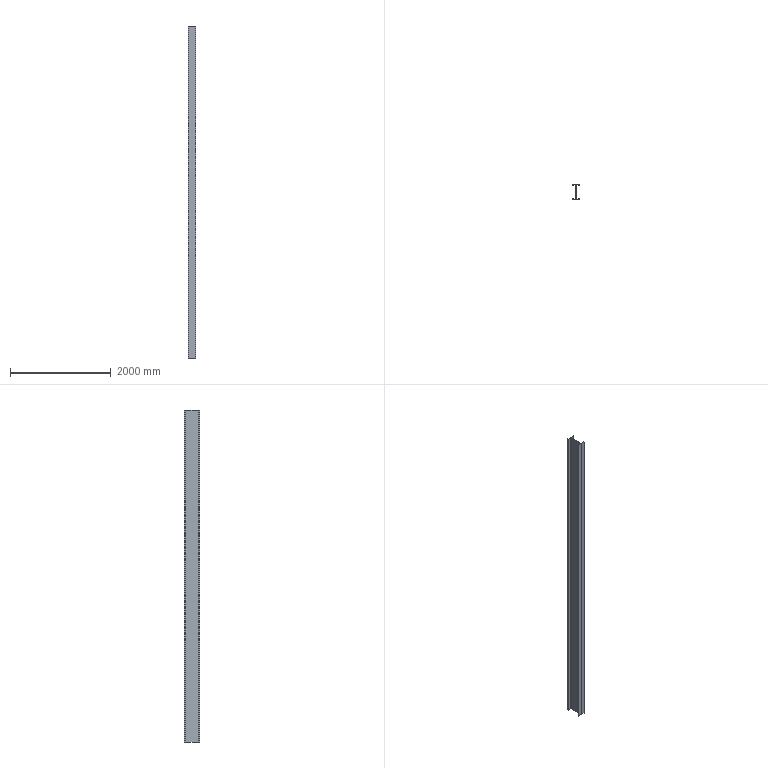Part | SolidWorks | features Extrusion 1 | 1 solid | 18 faces | box 150 x 300 x 6592 mm | volume 30837843 mm3 | plane 14 | cylinder 4 | commonest cylinder face diameters 26 x4
STEP:
#1=CARTESIAN_POINT('',(-75.,9.,0.));
#2=VERTEX_POINT('',#1);
#3=CARTESIAN_POINT('',(-75.,0.,0.));
#4=VERTEX_POINT('',#3);
#5=CARTESIAN_POINT('',(-75.,0.,0.));
#6=DIRECTION('',(0.,-1.,0.));
#7=VECTOR('',#6,1000.);
#8=LINE('',#5,#7);
#9=EDGE_CURVE('',#2,#4,#8,.T.);
#10=ORIENTED_EDGE('',*,*,#9,.T.);
#11=CARTESIAN_POINT('',(-75.,0.,6592.));
#12=VERTEX_POINT('',#11);
#13=CARTESIAN_POINT('',(-75.,0.,6592.));
#14=DIRECTION('',(0.,0.,-1.));
#15=VECTOR('',#14,1000.);
#16=LINE('',#13,#15);
#17=EDGE_CURVE('',#12,#4,#16,.T.);
#18=ORIENTED_EDGE('',*,*,#17,.F.);
#19=CARTESIAN_POINT('',(-75.,9.,6592.));
#20=VERTEX_POINT('',#19);
#21=CARTESIAN_POINT('',(-75.,0.,6592.));
#22=DIRECTION('',(0.,-1.,0.));
#23=VECTOR('',#22,1000.);
#24=LINE('',#21,#23);
#25=EDGE_CURVE('',#20,#12,#24,.T.);
#26=ORIENTED_EDGE('',*,*,#25,.F.);
#27=CARTESIAN_POINT('',(-75.,9.,6592.));
#28=DIRECTION('',(0.,0.,-1.));
#29=VECTOR('',#28,1000.);
#30=LINE('',#27,#29);
#31=EDGE_CURVE('',#20,#2,#30,.T.);
#32=ORIENTED_EDGE('',*,*,#31,.T.);
#33=EDGE_LOOP('',(#10,#18,#26,#32));
#34=FACE_OUTER_BOUND('',#33,.T.);
#35=CARTESIAN_POINT('',(-75.,0.,6592.));
#36=DIRECTION('',(1.,0.,0.));
#37=DIRECTION('',(0.,0.,-1.));
#38=AXIS2_PLACEMENT_3D('',#35,#36,#37);
#39=PLANE('',#38);
#40=ADVANCED_FACE('',(#34),#39,.F.);
#41=CARTESIAN_POINT('',(75.,0.,0.));
#42=VERTEX_POINT('',#41);
#43=CARTESIAN_POINT('',(75.,0.,0.));
#44=DIRECTION('',(1.,0.,0.));
#45=VECTOR('',#44,1000.);
#46=LINE('',#43,#45);
#47=EDGE_CURVE('',#4,#42,#46,.T.);
#48=ORIENTED_EDGE('',*,*,#47,.T.);
#49=CARTESIAN_POINT('',(75.,0.,6592.));
#50=VERTEX_POINT('',#49);
#51=CARTESIAN_POINT('',(75.,0.,6592.));
#52=DIRECTION('',(0.,0.,-1.));
#53=VECTOR('',#52,1000.);
#54=LINE('',#51,#53);
#55=EDGE_CURVE('',#50,#42,#54,.T.);
#56=ORIENTED_EDGE('',*,*,#55,.F.);
#57=CARTESIAN_POINT('',(75.,0.,6592.));
#58=DIRECTION('',(1.,0.,0.));
#59=VECTOR('',#58,1000.);
#60=LINE('',#57,#59);
#61=EDGE_CURVE('',#12,#50,#60,.T.);
#62=ORIENTED_EDGE('',*,*,#61,.F.);
#63=ORIENTED_EDGE('',*,*,#17,.T.);
#64=EDGE_LOOP('',(#48,#56,#62,#63));
#65=FACE_OUTER_BOUND('',#64,.T.);
#66=CARTESIAN_POINT('',(75.,0.,6592.));
#67=DIRECTION('',(0.,1.,0.));
#68=DIRECTION('',(-1.,0.,0.));
#69=AXIS2_PLACEMENT_3D('',#66,#67,#68);
#70=PLANE('',#69);
#71=ADVANCED_FACE('',(#65),#70,.F.);
#72=CARTESIAN_POINT('',(75.,9.,0.));
#73=VERTEX_POINT('',#72);
#74=CARTESIAN_POINT('',(75.,0.,0.));
#75=DIRECTION('',(0.,1.,0.));
#76=VECTOR('',#75,1000.);
#77=LINE('',#74,#76);
#78=EDGE_CURVE('',#42,#73,#77,.T.);
#79=ORIENTED_EDGE('',*,*,#78,.T.);
#80=CARTESIAN_POINT('',(75.,9.,6592.));
#81=VERTEX_POINT('',#80);
#82=CARTESIAN_POINT('',(75.,9.,6592.));
#83=DIRECTION('',(0.,0.,-1.));
#84=VECTOR('',#83,1000.);
#85=LINE('',#82,#84);
#86=EDGE_CURVE('',#81,#73,#85,.T.);
#87=ORIENTED_EDGE('',*,*,#86,.F.);
#88=CARTESIAN_POINT('',(75.,0.,6592.));
#89=DIRECTION('',(0.,1.,0.));
#90=VECTOR('',#89,1000.);
#91=LINE('',#88,#90);
#92=EDGE_CURVE('',#50,#81,#91,.T.);
#93=ORIENTED_EDGE('',*,*,#92,.F.);
#94=ORIENTED_EDGE('',*,*,#55,.T.);
#95=EDGE_LOOP('',(#79,#87,#93,#94));
#96=FACE_OUTER_BOUND('',#95,.T.);
#97=CARTESIAN_POINT('',(75.,0.,6592.));
#98=DIRECTION('',(-1.,0.,0.));
#99=DIRECTION('',(0.,0.,1.));
#100=AXIS2_PLACEMENT_3D('',#97,#98,#99);
#101=PLANE('',#100);
#102=ADVANCED_FACE('',(#96),#101,.F.);
#103=CARTESIAN_POINT('',(16.25,9.,0.));
#104=VERTEX_POINT('',#103);
#105=CARTESIAN_POINT('',(75.,9.,0.));
#106=DIRECTION('',(-1.,0.,0.));
#107=VECTOR('',#106,1000.);
#108=LINE('',#105,#107);
#109=EDGE_CURVE('',#73,#104,#108,.T.);
#110=ORIENTED_EDGE('',*,*,#109,.T.);
#111=CARTESIAN_POINT('',(16.25,9.,6592.));
#112=VERTEX_POINT('',#111);
#113=CARTESIAN_POINT('',(16.25,9.,6592.));
#114=DIRECTION('',(0.,0.,-1.));
#115=VECTOR('',#114,1000.);
#116=LINE('',#113,#115);
#117=EDGE_CURVE('',#112,#104,#116,.T.);
#118=ORIENTED_EDGE('',*,*,#117,.F.);
#119=CARTESIAN_POINT('',(75.,9.,6592.));
#120=DIRECTION('',(-1.,0.,0.));
#121=VECTOR('',#120,1000.);
#122=LINE('',#119,#121);
#123=EDGE_CURVE('',#81,#112,#122,.T.);
#124=ORIENTED_EDGE('',*,*,#123,.F.);
#125=ORIENTED_EDGE('',*,*,#86,.T.);
#126=EDGE_LOOP('',(#110,#118,#124,#125));
#127=FACE_OUTER_BOUND('',#126,.T.);
#128=CARTESIAN_POINT('',(75.,9.,6592.));
#129=DIRECTION('',(0.,-1.,0.));
#130=DIRECTION('',(1.,0.,0.));
#131=AXIS2_PLACEMENT_3D('',#128,#129,#130);
#132=PLANE('',#131);
#133=ADVANCED_FACE('',(#127),#132,.F.);
#134=CARTESIAN_POINT('',(3.25,22.,0.));
#135=VERTEX_POINT('',#134);
#136=CARTESIAN_POINT('',(16.25,22.,0.));
#137=DIRECTION('',(0.,0.,-1.));
#138=DIRECTION('',(-1.,0.,0.));
#139=AXIS2_PLACEMENT_3D('',#136,#137,#138);
#140=CIRCLE('',#139,13.);
#141=EDGE_CURVE('',#104,#135,#140,.T.);
#142=ORIENTED_EDGE('',*,*,#141,.T.);
#143=CARTESIAN_POINT('',(3.25,22.,6592.));
#144=VERTEX_POINT('',#143);
#145=CARTESIAN_POINT('',(3.25,22.,6592.));
#146=DIRECTION('',(0.,0.,-1.));
#147=VECTOR('',#146,1000.);
#148=LINE('',#145,#147);
#149=EDGE_CURVE('',#144,#135,#148,.T.);
#150=ORIENTED_EDGE('',*,*,#149,.F.);
#151=CARTESIAN_POINT('',(16.25,22.,6592.));
#152=DIRECTION('',(0.,0.,-1.));
#153=DIRECTION('',(-1.,0.,0.));
#154=AXIS2_PLACEMENT_3D('',#151,#152,#153);
#155=CIRCLE('',#154,13.);
#156=EDGE_CURVE('',#112,#144,#155,.T.);
#157=ORIENTED_EDGE('',*,*,#156,.F.);
#158=ORIENTED_EDGE('',*,*,#117,.T.);
#159=EDGE_LOOP('',(#142,#150,#157,#158));
#160=FACE_OUTER_BOUND('',#159,.T.);
#161=CARTESIAN_POINT('',(16.25,22.,6592.));
#162=DIRECTION('',(0.,0.,-1.));
#163=DIRECTION('',(-1.,0.,0.));
#164=AXIS2_PLACEMENT_3D('',#161,#162,#163);
#165=CYLINDRICAL_SURFACE('',#164,13.);
#166=ADVANCED_FACE('',(#160),#165,.F.);
#167=CARTESIAN_POINT('',(3.25,278.,0.));
#168=VERTEX_POINT('',#167);
#169=CARTESIAN_POINT('',(3.25,22.,0.));
#170=DIRECTION('',(0.,1.,0.));
#171=VECTOR('',#170,1000.);
#172=LINE('',#169,#171);
#173=EDGE_CURVE('',#135,#168,#172,.T.);
#174=ORIENTED_EDGE('',*,*,#173,.T.);
#175=CARTESIAN_POINT('',(3.25,278.,6592.));
#176=VERTEX_POINT('',#175);
#177=CARTESIAN_POINT('',(3.25,278.,6592.));
#178=DIRECTION('',(0.,0.,-1.));
#179=VECTOR('',#178,1000.);
#180=LINE('',#177,#179);
#181=EDGE_CURVE('',#176,#168,#180,.T.);
#182=ORIENTED_EDGE('',*,*,#181,.F.);
#183=CARTESIAN_POINT('',(3.25,22.,6592.));
#184=DIRECTION('',(0.,1.,0.));
#185=VECTOR('',#184,1000.);
#186=LINE('',#183,#185);
#187=EDGE_CURVE('',#144,#176,#186,.T.);
#188=ORIENTED_EDGE('',*,*,#187,.F.);
#189=ORIENTED_EDGE('',*,*,#149,.T.);
#190=EDGE_LOOP('',(#174,#182,#188,#189));
#191=FACE_OUTER_BOUND('',#190,.T.);
#192=CARTESIAN_POINT('',(3.25,22.,6592.));
#193=DIRECTION('',(-1.,0.,0.));
#194=DIRECTION('',(0.,0.,1.));
#195=AXIS2_PLACEMENT_3D('',#192,#193,#194);
#196=PLANE('',#195);
#197=ADVANCED_FACE('',(#191),#196,.F.);
#198=CARTESIAN_POINT('',(16.25,291.,0.));
#199=VERTEX_POINT('',#198);
#200=CARTESIAN_POINT('',(16.25,278.,0.));
#201=DIRECTION('',(0.,0.,-1.));
#202=DIRECTION('',(-1.,0.,0.));
#203=AXIS2_PLACEMENT_3D('',#200,#201,#202);
#204=CIRCLE('',#203,13.);
#205=EDGE_CURVE('',#168,#199,#204,.T.);
#206=ORIENTED_EDGE('',*,*,#205,.T.);
#207=CARTESIAN_POINT('',(16.25,291.,6592.));
#208=VERTEX_POINT('',#207);
#209=CARTESIAN_POINT('',(16.25,291.,6592.));
#210=DIRECTION('',(0.,0.,-1.));
#211=VECTOR('',#210,1000.);
#212=LINE('',#209,#211);
#213=EDGE_CURVE('',#208,#199,#212,.T.);
#214=ORIENTED_EDGE('',*,*,#213,.F.);
#215=CARTESIAN_POINT('',(16.25,278.,6592.));
#216=DIRECTION('',(0.,0.,-1.));
#217=DIRECTION('',(-1.,0.,0.));
#218=AXIS2_PLACEMENT_3D('',#215,#216,#217);
#219=CIRCLE('',#218,13.);
#220=EDGE_CURVE('',#176,#208,#219,.T.);
#221=ORIENTED_EDGE('',*,*,#220,.F.);
#222=ORIENTED_EDGE('',*,*,#181,.T.);
#223=EDGE_LOOP('',(#206,#214,#221,#222));
#224=FACE_OUTER_BOUND('',#223,.T.);
#225=CARTESIAN_POINT('',(16.25,278.,6592.));
#226=DIRECTION('',(0.,0.,-1.));
#227=DIRECTION('',(-1.,0.,0.));
#228=AXIS2_PLACEMENT_3D('',#225,#226,#227);
#229=CYLINDRICAL_SURFACE('',#228,13.);
#230=ADVANCED_FACE('',(#224),#229,.F.);
#231=CARTESIAN_POINT('',(75.,291.,0.));
#232=VERTEX_POINT('',#231);
#233=CARTESIAN_POINT('',(16.25,291.,0.));
#234=DIRECTION('',(1.,0.,0.));
#235=VECTOR('',#234,1000.);
#236=LINE('',#233,#235);
#237=EDGE_CURVE('',#199,#232,#236,.T.);
#238=ORIENTED_EDGE('',*,*,#237,.T.);
#239=CARTESIAN_POINT('',(75.,291.,6592.));
#240=VERTEX_POINT('',#239);
#241=CARTESIAN_POINT('',(75.,291.,6592.));
#242=DIRECTION('',(0.,0.,-1.));
#243=VECTOR('',#242,1000.);
#244=LINE('',#241,#243);
#245=EDGE_CURVE('',#240,#232,#244,.T.);
#246=ORIENTED_EDGE('',*,*,#245,.F.);
#247=CARTESIAN_POINT('',(16.25,291.,6592.));
#248=DIRECTION('',(1.,0.,0.));
#249=VECTOR('',#248,1000.);
#250=LINE('',#247,#249);
#251=EDGE_CURVE('',#208,#240,#250,.T.);
#252=ORIENTED_EDGE('',*,*,#251,.F.);
#253=ORIENTED_EDGE('',*,*,#213,.T.);
#254=EDGE_LOOP('',(#238,#246,#252,#253));
#255=FACE_OUTER_BOUND('',#254,.T.);
#256=CARTESIAN_POINT('',(16.25,291.,6592.));
#257=DIRECTION('',(0.,1.,0.));
#258=DIRECTION('',(-1.,0.,0.));
#259=AXIS2_PLACEMENT_3D('',#256,#257,#258);
#260=PLANE('',#259);
#261=ADVANCED_FACE('',(#255),#260,.F.);
#262=CARTESIAN_POINT('',(75.,300.,0.));
#263=VERTEX_POINT('',#262);
#264=CARTESIAN_POINT('',(75.,291.,0.));
#265=DIRECTION('',(0.,1.,0.));
#266=VECTOR('',#265,1000.);
#267=LINE('',#264,#266);
#268=EDGE_CURVE('',#232,#263,#267,.T.);
#269=ORIENTED_EDGE('',*,*,#268,.T.);
#270=CARTESIAN_POINT('',(75.,300.,6592.));
#271=VERTEX_POINT('',#270);
#272=CARTESIAN_POINT('',(75.,300.,6592.));
#273=DIRECTION('',(0.,0.,-1.));
#274=VECTOR('',#273,1000.);
#275=LINE('',#272,#274);
#276=EDGE_CURVE('',#271,#263,#275,.T.);
#277=ORIENTED_EDGE('',*,*,#276,.F.);
#278=CARTESIAN_POINT('',(75.,291.,6592.));
#279=DIRECTION('',(0.,1.,0.));
#280=VECTOR('',#279,1000.);
#281=LINE('',#278,#280);
#282=EDGE_CURVE('',#240,#271,#281,.T.);
#283=ORIENTED_EDGE('',*,*,#282,.F.);
#284=ORIENTED_EDGE('',*,*,#245,.T.);
#285=EDGE_LOOP('',(#269,#277,#283,#284));
#286=FACE_OUTER_BOUND('',#285,.T.);
#287=CARTESIAN_POINT('',(75.,291.,6592.));
#288=DIRECTION('',(-1.,0.,0.));
#289=DIRECTION('',(0.,-1.,0.));
#290=AXIS2_PLACEMENT_3D('',#287,#288,#289);
#291=PLANE('',#290);
#292=ADVANCED_FACE('',(#286),#291,.F.);
#293=CARTESIAN_POINT('',(-75.,300.,0.));
#294=VERTEX_POINT('',#293);
#295=CARTESIAN_POINT('',(-75.,300.,0.));
#296=DIRECTION('',(-1.,0.,0.));
#297=VECTOR('',#296,1000.);
#298=LINE('',#295,#297);
#299=EDGE_CURVE('',#263,#294,#298,.T.);
#300=ORIENTED_EDGE('',*,*,#299,.T.);
#301=CARTESIAN_POINT('',(-75.,300.,6592.));
#302=VERTEX_POINT('',#301);
#303=CARTESIAN_POINT('',(-75.,300.,6592.));
#304=DIRECTION('',(0.,0.,-1.));
#305=VECTOR('',#304,1000.);
#306=LINE('',#303,#305);
#307=EDGE_CURVE('',#302,#294,#306,.T.);
#308=ORIENTED_EDGE('',*,*,#307,.F.);
#309=CARTESIAN_POINT('',(-75.,300.,6592.));
#310=DIRECTION('',(-1.,0.,0.));
#311=VECTOR('',#310,1000.);
#312=LINE('',#309,#311);
#313=EDGE_CURVE('',#271,#302,#312,.T.);
#314=ORIENTED_EDGE('',*,*,#313,.F.);
#315=ORIENTED_EDGE('',*,*,#276,.T.);
#316=EDGE_LOOP('',(#300,#308,#314,#315));
#317=FACE_OUTER_BOUND('',#316,.T.);
#318=CARTESIAN_POINT('',(-75.,300.,6592.));
#319=DIRECTION('',(0.,-1.,0.));
#320=DIRECTION('',(0.,0.,-1.));
#321=AXIS2_PLACEMENT_3D('',#318,#319,#320);
#322=PLANE('',#321);
#323=ADVANCED_FACE('',(#317),#322,.F.);
#324=CARTESIAN_POINT('',(-75.,291.,0.));
#325=VERTEX_POINT('',#324);
#326=CARTESIAN_POINT('',(-75.,291.,0.));
#327=DIRECTION('',(0.,-1.,0.));
#328=VECTOR('',#327,1000.);
#329=LINE('',#326,#328);
#330=EDGE_CURVE('',#294,#325,#329,.T.);
#331=ORIENTED_EDGE('',*,*,#330,.T.);
#332=CARTESIAN_POINT('',(-75.,291.,6592.));
#333=VERTEX_POINT('',#332);
#334=CARTESIAN_POINT('',(-75.,291.,6592.));
#335=DIRECTION('',(0.,0.,-1.));
#336=VECTOR('',#335,1000.);
#337=LINE('',#334,#336);
#338=EDGE_CURVE('',#333,#325,#337,.T.);
#339=ORIENTED_EDGE('',*,*,#338,.F.);
#340=CARTESIAN_POINT('',(-75.,291.,6592.));
#341=DIRECTION('',(0.,-1.,0.));
#342=VECTOR('',#341,1000.);
#343=LINE('',#340,#342);
#344=EDGE_CURVE('',#302,#333,#343,.T.);
#345=ORIENTED_EDGE('',*,*,#344,.F.);
#346=ORIENTED_EDGE('',*,*,#307,.T.);
#347=EDGE_LOOP('',(#331,#339,#345,#346));
#348=FACE_OUTER_BOUND('',#347,.T.);
#349=CARTESIAN_POINT('',(-75.,291.,6592.));
#350=DIRECTION('',(1.,0.,0.));
#351=DIRECTION('',(0.,1.,0.));
#352=AXIS2_PLACEMENT_3D('',#349,#350,#351);
#353=PLANE('',#352);
#354=ADVANCED_FACE('',(#348),#353,.F.);
#355=CARTESIAN_POINT('',(-16.25,291.,0.));
#356=VERTEX_POINT('',#355);
#357=CARTESIAN_POINT('',(-16.25,291.,0.));
#358=DIRECTION('',(1.,0.,0.));
#359=VECTOR('',#358,1000.);
#360=LINE('',#357,#359);
#361=EDGE_CURVE('',#325,#356,#360,.T.);
#362=ORIENTED_EDGE('',*,*,#361,.T.);
#363=CARTESIAN_POINT('',(-16.25,291.,6592.));
#364=VERTEX_POINT('',#363);
#365=CARTESIAN_POINT('',(-16.25,291.,6592.));
#366=DIRECTION('',(0.,0.,-1.));
#367=VECTOR('',#366,1000.);
#368=LINE('',#365,#367);
#369=EDGE_CURVE('',#364,#356,#368,.T.);
#370=ORIENTED_EDGE('',*,*,#369,.F.);
#371=CARTESIAN_POINT('',(-16.25,291.,6592.));
#372=DIRECTION('',(1.,0.,0.));
#373=VECTOR('',#372,1000.);
#374=LINE('',#371,#373);
#375=EDGE_CURVE('',#333,#364,#374,.T.);
#376=ORIENTED_EDGE('',*,*,#375,.F.);
#377=ORIENTED_EDGE('',*,*,#338,.T.);
#378=EDGE_LOOP('',(#362,#370,#376,#377));
#379=FACE_OUTER_BOUND('',#378,.T.);
#380=CARTESIAN_POINT('',(-16.25,291.,6592.));
#381=DIRECTION('',(0.,1.,0.));
#382=DIRECTION('',(-1.,0.,0.));
#383=AXIS2_PLACEMENT_3D('',#380,#381,#382);
#384=PLANE('',#383);
#385=ADVANCED_FACE('',(#379),#384,.F.);
#386=CARTESIAN_POINT('',(-3.25,278.,0.));
#387=VERTEX_POINT('',#386);
#388=CARTESIAN_POINT('',(-16.25,278.,0.));
#389=DIRECTION('',(0.,0.,-1.));
#390=DIRECTION('',(1.,0.,0.));
#391=AXIS2_PLACEMENT_3D('',#388,#389,#390);
#392=CIRCLE('',#391,13.);
#393=EDGE_CURVE('',#356,#387,#392,.T.);
#394=ORIENTED_EDGE('',*,*,#393,.T.);
#395=CARTESIAN_POINT('',(-3.25,278.,6592.));
#396=VERTEX_POINT('',#395);
#397=CARTESIAN_POINT('',(-3.25,278.,6592.));
#398=DIRECTION('',(0.,0.,-1.));
#399=VECTOR('',#398,1000.);
#400=LINE('',#397,#399);
#401=EDGE_CURVE('',#396,#387,#400,.T.);
#402=ORIENTED_EDGE('',*,*,#401,.F.);
#403=CARTESIAN_POINT('',(-16.25,278.,6592.));
#404=DIRECTION('',(0.,0.,-1.));
#405=DIRECTION('',(1.,0.,0.));
#406=AXIS2_PLACEMENT_3D('',#403,#404,#405);
#407=CIRCLE('',#406,13.);
#408=EDGE_CURVE('',#364,#396,#407,.T.);
#409=ORIENTED_EDGE('',*,*,#408,.F.);
#410=ORIENTED_EDGE('',*,*,#369,.T.);
#411=EDGE_LOOP('',(#394,#402,#409,#410));
#412=FACE_OUTER_BOUND('',#411,.T.);
#413=CARTESIAN_POINT('',(-16.25,278.,6592.));
#414=DIRECTION('',(0.,0.,-1.));
#415=DIRECTION('',(-1.,0.,0.));
#416=AXIS2_PLACEMENT_3D('',#413,#414,#415);
#417=CYLINDRICAL_SURFACE('',#416,13.);
#418=ADVANCED_FACE('',(#412),#417,.F.);
#419=CARTESIAN_POINT('',(-3.25,22.,0.));
#420=VERTEX_POINT('',#419);
#421=CARTESIAN_POINT('',(-3.25,22.,0.));
#422=DIRECTION('',(0.,-1.,0.));
#423=VECTOR('',#422,1000.);
#424=LINE('',#421,#423);
#425=EDGE_CURVE('',#387,#420,#424,.T.);
#426=ORIENTED_EDGE('',*,*,#425,.T.);
#427=CARTESIAN_POINT('',(-3.25,22.,6592.));
#428=VERTEX_POINT('',#427);
#429=CARTESIAN_POINT('',(-3.25,22.,6592.));
#430=DIRECTION('',(0.,0.,-1.));
#431=VECTOR('',#430,1000.);
#432=LINE('',#429,#431);
#433=EDGE_CURVE('',#428,#420,#432,.T.);
#434=ORIENTED_EDGE('',*,*,#433,.F.);
#435=CARTESIAN_POINT('',(-3.25,22.,6592.));
#436=DIRECTION('',(0.,-1.,0.));
#437=VECTOR('',#436,1000.);
#438=LINE('',#435,#437);
#439=EDGE_CURVE('',#396,#428,#438,.T.);
#440=ORIENTED_EDGE('',*,*,#439,.F.);
#441=ORIENTED_EDGE('',*,*,#401,.T.);
#442=EDGE_LOOP('',(#426,#434,#440,#441));
#443=FACE_OUTER_BOUND('',#442,.T.);
#444=CARTESIAN_POINT('',(-3.25,22.,6592.));
#445=DIRECTION('',(1.,0.,0.));
#446=DIRECTION('',(0.,0.,-1.));
#447=AXIS2_PLACEMENT_3D('',#444,#445,#446);
#448=PLANE('',#447);
#449=ADVANCED_FACE('',(#443),#448,.F.);
#450=CARTESIAN_POINT('',(-16.25,9.,0.));
#451=VERTEX_POINT('',#450);
#452=CARTESIAN_POINT('',(-16.25,22.,0.));
#453=DIRECTION('',(0.,0.,-1.));
#454=DIRECTION('',(-1.,0.,0.));
#455=AXIS2_PLACEMENT_3D('',#452,#453,#454);
#456=CIRCLE('',#455,13.);
#457=EDGE_CURVE('',#420,#451,#456,.T.);
#458=ORIENTED_EDGE('',*,*,#457,.T.);
#459=CARTESIAN_POINT('',(-16.25,9.,6592.));
#460=VERTEX_POINT('',#459);
#461=CARTESIAN_POINT('',(-16.25,9.,6592.));
#462=DIRECTION('',(0.,0.,-1.));
#463=VECTOR('',#462,1000.);
#464=LINE('',#461,#463);
#465=EDGE_CURVE('',#460,#451,#464,.T.);
#466=ORIENTED_EDGE('',*,*,#465,.F.);
#467=CARTESIAN_POINT('',(-16.25,22.,6592.));
#468=DIRECTION('',(0.,0.,-1.));
#469=DIRECTION('',(-1.,0.,0.));
#470=AXIS2_PLACEMENT_3D('',#467,#468,#469);
#471=CIRCLE('',#470,13.);
#472=EDGE_CURVE('',#428,#460,#471,.T.);
#473=ORIENTED_EDGE('',*,*,#472,.F.);
#474=ORIENTED_EDGE('',*,*,#433,.T.);
#475=EDGE_LOOP('',(#458,#466,#473,#474));
#476=FACE_OUTER_BOUND('',#475,.T.);
#477=CARTESIAN_POINT('',(-16.25,22.,6592.));
#478=DIRECTION('',(0.,0.,-1.));
#479=DIRECTION('',(-1.,0.,0.));
#480=AXIS2_PLACEMENT_3D('',#477,#478,#479);
#481=CYLINDRICAL_SURFACE('',#480,13.);
#482=ADVANCED_FACE('',(#476),#481,.F.);
#483=CARTESIAN_POINT('',(-75.,9.,0.));
#484=DIRECTION('',(-1.,0.,0.));
#485=VECTOR('',#484,1000.);
#486=LINE('',#483,#485);
#487=EDGE_CURVE('',#451,#2,#486,.T.);
#488=ORIENTED_EDGE('',*,*,#487,.T.);
#489=ORIENTED_EDGE('',*,*,#31,.F.);
#490=CARTESIAN_POINT('',(-75.,9.,6592.));
#491=DIRECTION('',(-1.,0.,0.));
#492=VECTOR('',#491,1000.);
#493=LINE('',#490,#492);
#494=EDGE_CURVE('',#460,#20,#493,.T.);
#495=ORIENTED_EDGE('',*,*,#494,.F.);
#496=ORIENTED_EDGE('',*,*,#465,.T.);
#497=EDGE_LOOP('',(#488,#489,#495,#496));
#498=FACE_OUTER_BOUND('',#497,.T.);
#499=CARTESIAN_POINT('',(-75.,9.,6592.));
#500=DIRECTION('',(0.,-1.,0.));
#501=DIRECTION('',(1.,0.,0.));
#502=AXIS2_PLACEMENT_3D('',#499,#500,#501);
#503=PLANE('',#502);
#504=ADVANCED_FACE('',(#498),#503,.F.);
#505=ORIENTED_EDGE('',*,*,#25,.T.);
#506=ORIENTED_EDGE('',*,*,#61,.T.);
#507=ORIENTED_EDGE('',*,*,#92,.T.);
#508=ORIENTED_EDGE('',*,*,#123,.T.);
#509=ORIENTED_EDGE('',*,*,#156,.T.);
#510=ORIENTED_EDGE('',*,*,#187,.T.);
#511=ORIENTED_EDGE('',*,*,#220,.T.);
#512=ORIENTED_EDGE('',*,*,#251,.T.);
#513=ORIENTED_EDGE('',*,*,#282,.T.);
#514=ORIENTED_EDGE('',*,*,#313,.T.);
#515=ORIENTED_EDGE('',*,*,#344,.T.);
#516=ORIENTED_EDGE('',*,*,#375,.T.);
#517=ORIENTED_EDGE('',*,*,#408,.T.);
#518=ORIENTED_EDGE('',*,*,#439,.T.);
#519=ORIENTED_EDGE('',*,*,#472,.T.);
#520=ORIENTED_EDGE('',*,*,#494,.T.);
#521=EDGE_LOOP('',(#505,#506,#507,#508,#509,#510,#511,#512,#513,#514,#515,#516,#517,#518,#519,#520));
#522=FACE_OUTER_BOUND('',#521,.T.);
#523=CARTESIAN_POINT('',(-16.25,22.,6592.));
#524=DIRECTION('',(0.,0.,-1.));
#525=DIRECTION('',(-1.,0.,0.));
#526=AXIS2_PLACEMENT_3D('',#523,#524,#525);
#527=PLANE('',#526);
#528=ADVANCED_FACE('',(#522),#527,.F.);
#529=ORIENTED_EDGE('',*,*,#9,.F.);
#530=ORIENTED_EDGE('',*,*,#487,.F.);
#531=ORIENTED_EDGE('',*,*,#457,.F.);
#532=ORIENTED_EDGE('',*,*,#425,.F.);
#533=ORIENTED_EDGE('',*,*,#393,.F.);
#534=ORIENTED_EDGE('',*,*,#361,.F.);
#535=ORIENTED_EDGE('',*,*,#330,.F.);
#536=ORIENTED_EDGE('',*,*,#299,.F.);
#537=ORIENTED_EDGE('',*,*,#268,.F.);
#538=ORIENTED_EDGE('',*,*,#237,.F.);
#539=ORIENTED_EDGE('',*,*,#205,.F.);
#540=ORIENTED_EDGE('',*,*,#173,.F.);
#541=ORIENTED_EDGE('',*,*,#141,.F.);
#542=ORIENTED_EDGE('',*,*,#109,.F.);
#543=ORIENTED_EDGE('',*,*,#78,.F.);
#544=ORIENTED_EDGE('',*,*,#47,.F.);
#545=EDGE_LOOP('',(#529,#530,#531,#532,#533,#534,#535,#536,#537,#538,#539,#540,#541,#542,#543,#544));
#546=FACE_OUTER_BOUND('',#545,.T.);
#547=CARTESIAN_POINT('',(-16.25,22.,0.));
#548=DIRECTION('',(0.,0.,-1.));
#549=DIRECTION('',(-1.,0.,0.));
#550=AXIS2_PLACEMENT_3D('',#547,#548,#549);
#551=PLANE('',#550);
#552=ADVANCED_FACE('',(#546),#551,.T.);
#553=CLOSED_SHELL('',(#40,#71,#102,#133,#166,#197,#230,#261,#292,#323,#354,#385,#418,#449,#482,#504,#528,#552));
#554=MANIFOLD_SOLID_BREP('',#553);
#555=CARTESIAN_POINT('',(0.,0.,0.));
#556=DIRECTION('',(0.,0.,1.));
#557=DIRECTION('',(1.,0.,0.));
#558=AXIS2_PLACEMENT_3D('',#555,#556,#557);
#559=(LENGTH_UNIT()NAMED_UNIT(*)SI_UNIT(.MILLI.,.METRE.));
#560=UNCERTAINTY_MEASURE_WITH_UNIT(LENGTH_MEASURE(0.00001),#559,'','');
#561=(NAMED_UNIT(*)PLANE_ANGLE_UNIT()SI_UNIT($,.RADIAN.));
#562=(NAMED_UNIT(*)SI_UNIT($,.STERADIAN.)SOLID_ANGLE_UNIT());
#563=(GEOMETRIC_REPRESENTATION_CONTEXT(3)GLOBAL_UNCERTAINTY_ASSIGNED_CONTEXT((#560))GLOBAL_UNIT_ASSIGNED_CONTEXT((#559,#561,#562))REPRESENTATION_CONTEXT('',''));
#564=ADVANCED_BREP_SHAPE_REPRESENTATION('',(#554,#558),#563);